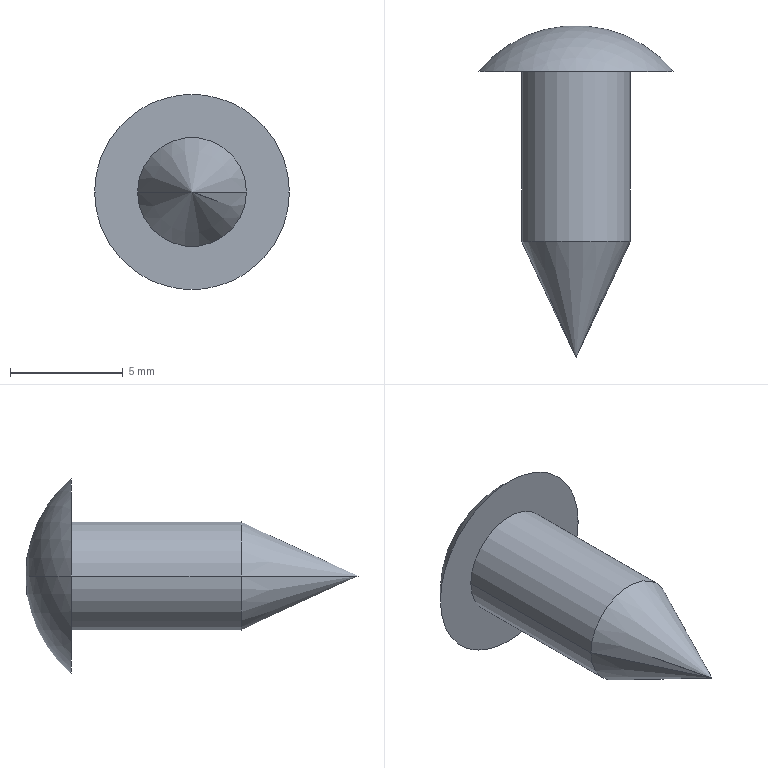Part | NX | features BREP 1 | 1 solid | 7 faces | box 8.636 x 14.732 x 8.636 mm | volume 233.112 mm3 | cone 2 | cylinder 2 | sphere 2 | plane 1 | commonest cylinder face diameters 4.826 x2
STEP:
#1=CARTESIAN_POINT('',(2.413,-7.525,0.));
#2=VERTEX_POINT('',#1);
#3=CARTESIAN_POINT('',(-2.413,-7.525,0.));
#4=VERTEX_POINT('',#3);
#5=CARTESIAN_POINT('',(0.,-7.525,0.));
#6=DIRECTION('',(0.,-1.,0.));
#7=DIRECTION('',(1.,0.,0.));
#8=AXIS2_PLACEMENT_3D('',#5,#6,#7);
#9=CIRCLE('',#8,2.413);
#10=EDGE_CURVE('',#2,#4,#9,.T.);
#11=ORIENTED_EDGE('',*,*,#10,.T.);
#12=CARTESIAN_POINT('',(0.,-12.7,0.));
#13=VERTEX_POINT('',#12);
#14=CARTESIAN_POINT('',(0.,-12.7,0.));
#15=DIRECTION('',(-0.4226,0.9063,0.));
#16=VECTOR('',#15,1000.);
#17=LINE('',#14,#16);
#18=EDGE_CURVE('',#4,#13,#17,.F.);
#19=ORIENTED_EDGE('',*,*,#18,.T.);
#20=CARTESIAN_POINT('',(0.,-12.7,0.));
#21=DIRECTION('',(0.4226,0.9063,0.));
#22=VECTOR('',#21,1000.);
#23=LINE('',#20,#22);
#24=EDGE_CURVE('',#2,#13,#23,.F.);
#25=ORIENTED_EDGE('',*,*,#24,.F.);
#26=EDGE_LOOP('',(#11,#19,#25));
#27=FACE_BOUND('',#26,.T.);
#28=CARTESIAN_POINT('',(0.,-10.061,0.));
#29=DIRECTION('',(0.,1.,0.));
#30=DIRECTION('',(1.,0.,0.));
#31=AXIS2_PLACEMENT_3D('',#28,#29,#30);
#32=CONICAL_SURFACE('',#31,1.231,0.4363);
#33=ADVANCED_FACE('',(#27),#32,.T.);
#34=ORIENTED_EDGE('',*,*,#18,.F.);
#35=CARTESIAN_POINT('',(0.,-7.525,0.));
#36=DIRECTION('',(0.,1.,0.));
#37=DIRECTION('',(1.,0.,0.));
#38=AXIS2_PLACEMENT_3D('',#35,#36,#37);
#39=CIRCLE('',#38,2.413);
#40=EDGE_CURVE('',#2,#4,#39,.T.);
#41=ORIENTED_EDGE('',*,*,#40,.F.);
#42=ORIENTED_EDGE('',*,*,#24,.T.);
#43=EDGE_LOOP('',(#34,#41,#42));
#44=FACE_BOUND('',#43,.T.);
#45=CARTESIAN_POINT('',(0.,-10.061,0.));
#46=DIRECTION('',(0.,1.,0.));
#47=DIRECTION('',(1.,0.,0.));
#48=AXIS2_PLACEMENT_3D('',#45,#46,#47);
#49=CONICAL_SURFACE('',#48,1.231,0.4363);
#50=ADVANCED_FACE('',(#44),#49,.T.);
#51=CARTESIAN_POINT('',(2.413,0.,0.));
#52=VERTEX_POINT('',#51);
#53=CARTESIAN_POINT('',(2.413,-7.525,0.));
#54=DIRECTION('',(0.,1.,0.));
#55=VECTOR('',#54,1000.);
#56=LINE('',#53,#55);
#57=EDGE_CURVE('',#52,#2,#56,.F.);
#58=ORIENTED_EDGE('',*,*,#57,.T.);
#59=ORIENTED_EDGE('',*,*,#40,.T.);
#60=CARTESIAN_POINT('',(-2.413,0.,0.));
#61=VERTEX_POINT('',#60);
#62=CARTESIAN_POINT('',(-2.413,-7.525,0.));
#63=DIRECTION('',(0.,1.,0.));
#64=VECTOR('',#63,1000.);
#65=LINE('',#62,#64);
#66=EDGE_CURVE('',#61,#4,#65,.F.);
#67=ORIENTED_EDGE('',*,*,#66,.F.);
#68=CARTESIAN_POINT('',(0.,0.,0.));
#69=DIRECTION('',(0.,-1.,0.));
#70=DIRECTION('',(-1.,0.,0.));
#71=AXIS2_PLACEMENT_3D('',#68,#69,#70);
#72=CIRCLE('',#71,2.413);
#73=EDGE_CURVE('',#61,#52,#72,.T.);
#74=ORIENTED_EDGE('',*,*,#73,.T.);
#75=EDGE_LOOP('',(#58,#59,#67,#74));
#76=FACE_BOUND('',#75,.T.);
#77=CARTESIAN_POINT('',(0.,0.635,0.));
#78=DIRECTION('',(0.,-1.,0.));
#79=DIRECTION('',(-1.,0.,0.));
#80=AXIS2_PLACEMENT_3D('',#77,#78,#79);
#81=CYLINDRICAL_SURFACE('',#80,2.413);
#82=ADVANCED_FACE('',(#76),#81,.T.);
#83=CARTESIAN_POINT('',(4.318,0.,0.));
#84=VERTEX_POINT('',#83);
#85=CARTESIAN_POINT('',(-4.318,0.,0.));
#86=VERTEX_POINT('',#85);
#87=CARTESIAN_POINT('',(0.,0.,0.));
#88=DIRECTION('',(0.,1.,0.));
#89=DIRECTION('',(1.,0.,0.));
#90=AXIS2_PLACEMENT_3D('',#87,#88,#89);
#91=CIRCLE('',#90,4.318);
#92=EDGE_CURVE('',#84,#86,#91,.T.);
#93=ORIENTED_EDGE('',*,*,#92,.F.);
#94=CARTESIAN_POINT('',(0.,0.,0.));
#95=DIRECTION('',(0.,-1.,0.));
#96=DIRECTION('',(1.,0.,0.));
#97=AXIS2_PLACEMENT_3D('',#94,#95,#96);
#98=CIRCLE('',#97,4.318);
#99=EDGE_CURVE('',#84,#86,#98,.T.);
#100=ORIENTED_EDGE('',*,*,#99,.T.);
#101=EDGE_LOOP('',(#93,#100));
#102=FACE_BOUND('',#101,.T.);
#103=ORIENTED_EDGE('',*,*,#73,.F.);
#104=CARTESIAN_POINT('',(0.,0.,0.));
#105=DIRECTION('',(0.,-1.,0.));
#106=DIRECTION('',(1.,0.,0.));
#107=AXIS2_PLACEMENT_3D('',#104,#105,#106);
#108=CIRCLE('',#107,2.413);
#109=EDGE_CURVE('',#52,#61,#108,.T.);
#110=ORIENTED_EDGE('',*,*,#109,.F.);
#111=EDGE_LOOP('',(#103,#110));
#112=FACE_BOUND('',#111,.T.);
#113=CARTESIAN_POINT('',(0.,0.,0.));
#114=DIRECTION('',(0.,-1.,0.));
#115=DIRECTION('',(0.,0.,-1.));
#116=AXIS2_PLACEMENT_3D('',#113,#114,#115);
#117=PLANE('',#116);
#118=ADVANCED_FACE('',(#102,#112),#117,.T.);
#119=CARTESIAN_POINT('',(0.,-3.572,0.));
#120=DIRECTION('',(0.,0.,-1.));
#121=DIRECTION('',(-0.7705,0.6374,0.));
#122=AXIS2_PLACEMENT_3D('',#119,#120,#121);
#123=CIRCLE('',#122,5.604);
#124=EDGE_CURVE('',#86,#84,#123,.T.);
#125=ORIENTED_EDGE('',*,*,#124,.F.);
#126=ORIENTED_EDGE('',*,*,#99,.F.);
#127=EDGE_LOOP('',(#125,#126));
#128=FACE_BOUND('',#127,.T.);
#129=CARTESIAN_POINT('',(0.,-3.572,0.));
#130=DIRECTION('',(0.,0.,-1.));
#131=DIRECTION('',(-1.,0.,0.));
#132=AXIS2_PLACEMENT_3D('',#129,#130,#131);
#133=SPHERICAL_SURFACE('',#132,5.604);
#134=ADVANCED_FACE('',(#128),#133,.T.);
#135=ORIENTED_EDGE('',*,*,#92,.T.);
#136=ORIENTED_EDGE('',*,*,#124,.T.);
#137=EDGE_LOOP('',(#135,#136));
#138=FACE_BOUND('',#137,.T.);
#139=CARTESIAN_POINT('',(0.,-3.572,0.));
#140=DIRECTION('',(0.,0.,-1.));
#141=DIRECTION('',(-1.,0.,0.));
#142=AXIS2_PLACEMENT_3D('',#139,#140,#141);
#143=SPHERICAL_SURFACE('',#142,5.604);
#144=ADVANCED_FACE('',(#138),#143,.T.);
#145=ORIENTED_EDGE('',*,*,#66,.T.);
#146=ORIENTED_EDGE('',*,*,#10,.F.);
#147=ORIENTED_EDGE('',*,*,#57,.F.);
#148=ORIENTED_EDGE('',*,*,#109,.T.);
#149=EDGE_LOOP('',(#145,#146,#147,#148));
#150=FACE_BOUND('',#149,.T.);
#151=CARTESIAN_POINT('',(0.,0.635,0.));
#152=DIRECTION('',(0.,-1.,0.));
#153=DIRECTION('',(-1.,0.,0.));
#154=AXIS2_PLACEMENT_3D('',#151,#152,#153);
#155=CYLINDRICAL_SURFACE('',#154,2.413);
#156=ADVANCED_FACE('',(#150),#155,.T.);
#157=CLOSED_SHELL('',(#33,#50,#82,#118,#134,#144,#156));
#158=MANIFOLD_SOLID_BREP('',#157);
#159=(LENGTH_UNIT()NAMED_UNIT(*)SI_UNIT(.MILLI.,.METRE.));
#160=UNCERTAINTY_MEASURE_WITH_UNIT(LENGTH_MEASURE(0.00001),#159,'','');
#161=(NAMED_UNIT(*)PLANE_ANGLE_UNIT()SI_UNIT($,.RADIAN.));
#162=(NAMED_UNIT(*)SI_UNIT($,.STERADIAN.)SOLID_ANGLE_UNIT());
#163=(GEOMETRIC_REPRESENTATION_CONTEXT(3)GLOBAL_UNCERTAINTY_ASSIGNED_CONTEXT((#160))GLOBAL_UNIT_ASSIGNED_CONTEXT((#159,#161,#162))REPRESENTATION_CONTEXT('',''));
#164=ADVANCED_BREP_SHAPE_REPRESENTATION('',(#158),#163);